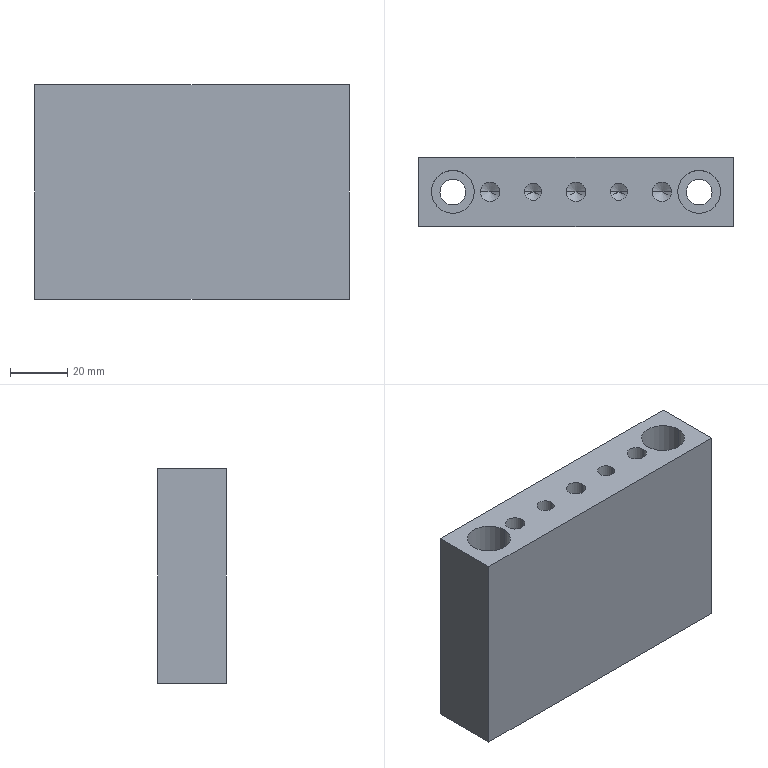Part | STEP file | PN_0026 | 1 solid | 44 faces | box 110 x 24 x 75 mm | volume 174240 mm3 | cylinder 22 | cone 14 | plane 8 | commonest cylinder face diameters 6 x8 6.8 x6 9 x4 15 x4